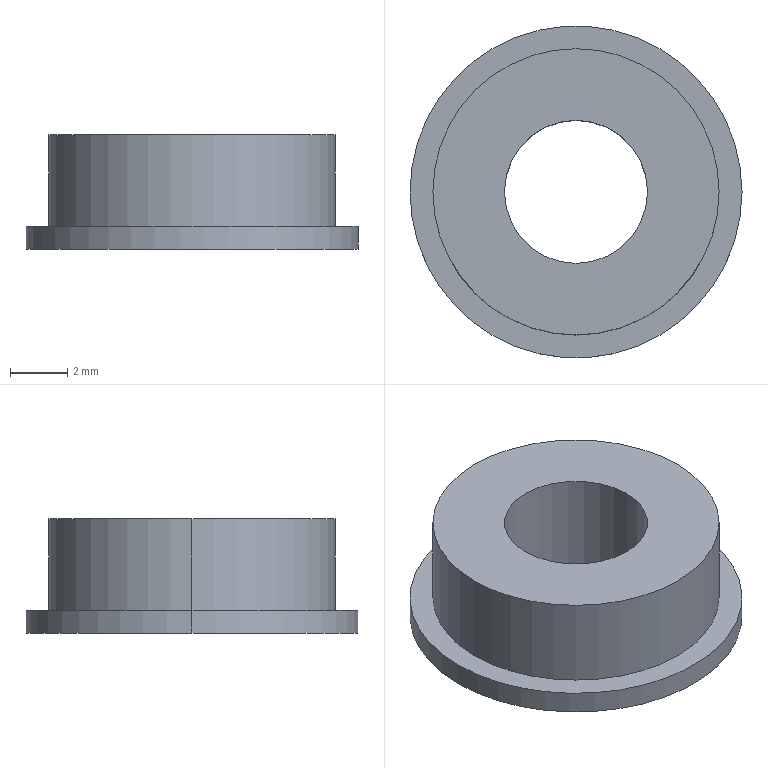Part | SolidWorks | features Extrusion 1, ICE 1 | 1 solid | 9 faces | box 11.6 x 11.6 x 4 mm | volume 257.334 mm3 | cylinder 6 | plane 3 | commonest cylinder face diameters 5 x2 10 x2 11.6 x2
STEP:
#1=CARTESIAN_POINT('',(5.,0.,4.));
#2=VERTEX_POINT('',#1);
#3=CARTESIAN_POINT('',(-5.,0.,4.));
#4=VERTEX_POINT('',#3);
#5=CARTESIAN_POINT('',(0.,0.,4.));
#6=DIRECTION('',(0.,0.,1.));
#7=DIRECTION('',(1.,0.,0.));
#8=AXIS2_PLACEMENT_3D('',#5,#6,#7);
#9=CIRCLE('',#8,5.);
#10=EDGE_CURVE('',#2,#4,#9,.T.);
#11=ORIENTED_EDGE('',*,*,#10,.F.);
#12=CARTESIAN_POINT('',(5.,0.,0.8));
#13=VERTEX_POINT('',#12);
#14=CARTESIAN_POINT('',(5.,0.,4.));
#15=DIRECTION('',(0.,0.,-1.));
#16=VECTOR('',#15,1000.);
#17=LINE('',#14,#16);
#18=EDGE_CURVE('',#2,#13,#17,.T.);
#19=ORIENTED_EDGE('',*,*,#18,.T.);
#20=CARTESIAN_POINT('',(-5.,0.,0.8));
#21=VERTEX_POINT('',#20);
#22=CARTESIAN_POINT('',(0.,0.,0.8));
#23=DIRECTION('',(0.,0.,1.));
#24=DIRECTION('',(1.,0.,0.));
#25=AXIS2_PLACEMENT_3D('',#22,#23,#24);
#26=CIRCLE('',#25,5.);
#27=EDGE_CURVE('',#13,#21,#26,.T.);
#28=ORIENTED_EDGE('',*,*,#27,.T.);
#29=CARTESIAN_POINT('',(-5.,0.,4.));
#30=DIRECTION('',(0.,0.,-1.));
#31=VECTOR('',#30,1000.);
#32=LINE('',#29,#31);
#33=EDGE_CURVE('',#4,#21,#32,.T.);
#34=ORIENTED_EDGE('',*,*,#33,.F.);
#35=EDGE_LOOP('',(#11,#19,#28,#34));
#36=FACE_OUTER_BOUND('',#35,.T.);
#37=CARTESIAN_POINT('',(0.,0.,4.));
#38=DIRECTION('',(0.,0.,-1.));
#39=DIRECTION('',(-1.,0.,0.));
#40=AXIS2_PLACEMENT_3D('',#37,#38,#39);
#41=CYLINDRICAL_SURFACE('',#40,5.);
#42=ADVANCED_FACE('',(#36),#41,.T.);
#43=CARTESIAN_POINT('',(-2.5,0.,4.));
#44=VERTEX_POINT('',#43);
#45=CARTESIAN_POINT('',(2.5,0.,4.));
#46=VERTEX_POINT('',#45);
#47=CARTESIAN_POINT('',(0.,0.,4.));
#48=DIRECTION('',(0.,0.,1.));
#49=DIRECTION('',(1.,0.,0.));
#50=AXIS2_PLACEMENT_3D('',#47,#48,#49);
#51=CIRCLE('',#50,2.5);
#52=EDGE_CURVE('',#44,#46,#51,.T.);
#53=ORIENTED_EDGE('',*,*,#52,.T.);
#54=CARTESIAN_POINT('',(2.5,0.,0.));
#55=VERTEX_POINT('',#54);
#56=CARTESIAN_POINT('',(2.5,0.,0.8));
#57=DIRECTION('',(0.,0.,-1.));
#58=VECTOR('',#57,1000.);
#59=LINE('',#56,#58);
#60=EDGE_CURVE('',#46,#55,#59,.T.);
#61=ORIENTED_EDGE('',*,*,#60,.T.);
#62=CARTESIAN_POINT('',(-2.5,0.,0.));
#63=VERTEX_POINT('',#62);
#64=CARTESIAN_POINT('',(0.,0.,0.));
#65=DIRECTION('',(0.,0.,1.));
#66=DIRECTION('',(1.,0.,0.));
#67=AXIS2_PLACEMENT_3D('',#64,#65,#66);
#68=CIRCLE('',#67,2.5);
#69=EDGE_CURVE('',#63,#55,#68,.T.);
#70=ORIENTED_EDGE('',*,*,#69,.F.);
#71=CARTESIAN_POINT('',(-2.5,0.,0.8));
#72=DIRECTION('',(0.,0.,-1.));
#73=VECTOR('',#72,1000.);
#74=LINE('',#71,#73);
#75=EDGE_CURVE('',#44,#63,#74,.T.);
#76=ORIENTED_EDGE('',*,*,#75,.F.);
#77=EDGE_LOOP('',(#53,#61,#70,#76));
#78=FACE_OUTER_BOUND('',#77,.T.);
#79=CARTESIAN_POINT('',(0.,0.,0.8));
#80=DIRECTION('',(0.,0.,-1.));
#81=DIRECTION('',(-1.,0.,0.));
#82=AXIS2_PLACEMENT_3D('',#79,#80,#81);
#83=CYLINDRICAL_SURFACE('',#82,2.5);
#84=ADVANCED_FACE('',(#78),#83,.F.);
#85=CARTESIAN_POINT('',(5.8,0.,0.8));
#86=VERTEX_POINT('',#85);
#87=CARTESIAN_POINT('',(-5.8,0.,0.8));
#88=VERTEX_POINT('',#87);
#89=CARTESIAN_POINT('',(0.,0.,0.8));
#90=DIRECTION('',(0.,0.,1.));
#91=DIRECTION('',(1.,0.,0.));
#92=AXIS2_PLACEMENT_3D('',#89,#90,#91);
#93=CIRCLE('',#92,5.8);
#94=EDGE_CURVE('',#86,#88,#93,.T.);
#95=ORIENTED_EDGE('',*,*,#94,.F.);
#96=CARTESIAN_POINT('',(5.8,0.,0.));
#97=VERTEX_POINT('',#96);
#98=CARTESIAN_POINT('',(5.8,0.,0.8));
#99=DIRECTION('',(0.,0.,-1.));
#100=VECTOR('',#99,1000.);
#101=LINE('',#98,#100);
#102=EDGE_CURVE('',#86,#97,#101,.T.);
#103=ORIENTED_EDGE('',*,*,#102,.T.);
#104=CARTESIAN_POINT('',(-5.8,0.,0.));
#105=VERTEX_POINT('',#104);
#106=CARTESIAN_POINT('',(0.,0.,0.));
#107=DIRECTION('',(0.,0.,1.));
#108=DIRECTION('',(1.,0.,0.));
#109=AXIS2_PLACEMENT_3D('',#106,#107,#108);
#110=CIRCLE('',#109,5.8);
#111=EDGE_CURVE('',#97,#105,#110,.T.);
#112=ORIENTED_EDGE('',*,*,#111,.T.);
#113=CARTESIAN_POINT('',(-5.8,0.,0.8));
#114=DIRECTION('',(0.,0.,-1.));
#115=VECTOR('',#114,1000.);
#116=LINE('',#113,#115);
#117=EDGE_CURVE('',#88,#105,#116,.T.);
#118=ORIENTED_EDGE('',*,*,#117,.F.);
#119=EDGE_LOOP('',(#95,#103,#112,#118));
#120=FACE_OUTER_BOUND('',#119,.T.);
#121=CARTESIAN_POINT('',(0.,0.,0.8));
#122=DIRECTION('',(0.,0.,-1.));
#123=DIRECTION('',(-1.,0.,0.));
#124=AXIS2_PLACEMENT_3D('',#121,#122,#123);
#125=CYLINDRICAL_SURFACE('',#124,5.8);
#126=ADVANCED_FACE('',(#120),#125,.T.);
#127=CARTESIAN_POINT('',(0.,0.,0.8));
#128=DIRECTION('',(0.,0.,1.));
#129=DIRECTION('',(1.,0.,0.));
#130=AXIS2_PLACEMENT_3D('',#127,#128,#129);
#131=CIRCLE('',#130,5.);
#132=EDGE_CURVE('',#21,#13,#131,.T.);
#133=ORIENTED_EDGE('',*,*,#132,.F.);
#134=ORIENTED_EDGE('',*,*,#27,.F.);
#135=EDGE_LOOP('',(#133,#134));
#136=FACE_BOUND('',#135,.T.);
#137=CARTESIAN_POINT('',(0.,0.,0.8));
#138=DIRECTION('',(0.,0.,1.));
#139=DIRECTION('',(1.,0.,0.));
#140=AXIS2_PLACEMENT_3D('',#137,#138,#139);
#141=CIRCLE('',#140,5.8);
#142=EDGE_CURVE('',#88,#86,#141,.T.);
#143=ORIENTED_EDGE('',*,*,#142,.T.);
#144=ORIENTED_EDGE('',*,*,#94,.T.);
#145=EDGE_LOOP('',(#143,#144));
#146=FACE_OUTER_BOUND('',#145,.T.);
#147=CARTESIAN_POINT('',(0.,0.,0.8));
#148=DIRECTION('',(0.,0.,1.));
#149=DIRECTION('',(1.,0.,0.));
#150=AXIS2_PLACEMENT_3D('',#147,#148,#149);
#151=PLANE('',#150);
#152=ADVANCED_FACE('',(#136,#146),#151,.T.);
#153=CARTESIAN_POINT('',(0.,0.,0.));
#154=DIRECTION('',(0.,0.,1.));
#155=DIRECTION('',(1.,0.,0.));
#156=AXIS2_PLACEMENT_3D('',#153,#154,#155);
#157=CIRCLE('',#156,5.8);
#158=EDGE_CURVE('',#105,#97,#157,.T.);
#159=ORIENTED_EDGE('',*,*,#158,.F.);
#160=ORIENTED_EDGE('',*,*,#111,.F.);
#161=EDGE_LOOP('',(#159,#160));
#162=FACE_OUTER_BOUND('',#161,.T.);
#163=ORIENTED_EDGE('',*,*,#69,.T.);
#164=CARTESIAN_POINT('',(0.,0.,0.));
#165=DIRECTION('',(0.,0.,1.));
#166=DIRECTION('',(1.,0.,0.));
#167=AXIS2_PLACEMENT_3D('',#164,#165,#166);
#168=CIRCLE('',#167,2.5);
#169=EDGE_CURVE('',#55,#63,#168,.T.);
#170=ORIENTED_EDGE('',*,*,#169,.T.);
#171=EDGE_LOOP('',(#163,#170));
#172=FACE_BOUND('',#171,.T.);
#173=CARTESIAN_POINT('',(0.,0.,0.));
#174=DIRECTION('',(0.,0.,1.));
#175=DIRECTION('',(1.,0.,0.));
#176=AXIS2_PLACEMENT_3D('',#173,#174,#175);
#177=PLANE('',#176);
#178=ADVANCED_FACE('',(#162,#172),#177,.F.);
#179=ORIENTED_EDGE('',*,*,#102,.F.);
#180=ORIENTED_EDGE('',*,*,#142,.F.);
#181=ORIENTED_EDGE('',*,*,#117,.T.);
#182=ORIENTED_EDGE('',*,*,#158,.T.);
#183=EDGE_LOOP('',(#179,#180,#181,#182));
#184=FACE_OUTER_BOUND('',#183,.T.);
#185=CARTESIAN_POINT('',(0.,0.,0.8));
#186=DIRECTION('',(0.,0.,-1.));
#187=DIRECTION('',(-1.,0.,0.));
#188=AXIS2_PLACEMENT_3D('',#185,#186,#187);
#189=CYLINDRICAL_SURFACE('',#188,5.8);
#190=ADVANCED_FACE('',(#184),#189,.T.);
#191=ORIENTED_EDGE('',*,*,#60,.F.);
#192=CARTESIAN_POINT('',(0.,0.,4.));
#193=DIRECTION('',(0.,0.,1.));
#194=DIRECTION('',(1.,0.,0.));
#195=AXIS2_PLACEMENT_3D('',#192,#193,#194);
#196=CIRCLE('',#195,2.5);
#197=EDGE_CURVE('',#46,#44,#196,.T.);
#198=ORIENTED_EDGE('',*,*,#197,.T.);
#199=ORIENTED_EDGE('',*,*,#75,.T.);
#200=ORIENTED_EDGE('',*,*,#169,.F.);
#201=EDGE_LOOP('',(#191,#198,#199,#200));
#202=FACE_OUTER_BOUND('',#201,.T.);
#203=CARTESIAN_POINT('',(0.,0.,0.8));
#204=DIRECTION('',(0.,0.,-1.));
#205=DIRECTION('',(-1.,0.,0.));
#206=AXIS2_PLACEMENT_3D('',#203,#204,#205);
#207=CYLINDRICAL_SURFACE('',#206,2.5);
#208=ADVANCED_FACE('',(#202),#207,.F.);
#209=CARTESIAN_POINT('',(0.,0.,4.));
#210=DIRECTION('',(0.,0.,1.));
#211=DIRECTION('',(1.,0.,0.));
#212=AXIS2_PLACEMENT_3D('',#209,#210,#211);
#213=CIRCLE('',#212,5.);
#214=EDGE_CURVE('',#4,#2,#213,.T.);
#215=ORIENTED_EDGE('',*,*,#214,.T.);
#216=ORIENTED_EDGE('',*,*,#10,.T.);
#217=EDGE_LOOP('',(#215,#216));
#218=FACE_OUTER_BOUND('',#217,.T.);
#219=ORIENTED_EDGE('',*,*,#52,.F.);
#220=ORIENTED_EDGE('',*,*,#197,.F.);
#221=EDGE_LOOP('',(#219,#220));
#222=FACE_BOUND('',#221,.T.);
#223=CARTESIAN_POINT('',(0.,0.,4.));
#224=DIRECTION('',(0.,0.,1.));
#225=DIRECTION('',(1.,0.,0.));
#226=AXIS2_PLACEMENT_3D('',#223,#224,#225);
#227=PLANE('',#226);
#228=ADVANCED_FACE('',(#218,#222),#227,.T.);
#229=ORIENTED_EDGE('',*,*,#18,.F.);
#230=ORIENTED_EDGE('',*,*,#214,.F.);
#231=ORIENTED_EDGE('',*,*,#33,.T.);
#232=ORIENTED_EDGE('',*,*,#132,.T.);
#233=EDGE_LOOP('',(#229,#230,#231,#232));
#234=FACE_OUTER_BOUND('',#233,.T.);
#235=CARTESIAN_POINT('',(0.,0.,4.));
#236=DIRECTION('',(0.,0.,-1.));
#237=DIRECTION('',(-1.,0.,0.));
#238=AXIS2_PLACEMENT_3D('',#235,#236,#237);
#239=CYLINDRICAL_SURFACE('',#238,5.);
#240=ADVANCED_FACE('',(#234),#239,.T.);
#241=CLOSED_SHELL('',(#42,#84,#126,#152,#178,#190,#208,#228,#240));
#242=MANIFOLD_SOLID_BREP('',#241);
#243=CARTESIAN_POINT('',(0.,0.,0.));
#244=DIRECTION('',(0.,0.,1.));
#245=DIRECTION('',(1.,0.,0.));
#246=AXIS2_PLACEMENT_3D('',#243,#244,#245);
#247=(LENGTH_UNIT()NAMED_UNIT(*)SI_UNIT(.MILLI.,.METRE.));
#248=UNCERTAINTY_MEASURE_WITH_UNIT(LENGTH_MEASURE(0.00001),#247,'','');
#249=(NAMED_UNIT(*)PLANE_ANGLE_UNIT()SI_UNIT($,.RADIAN.));
#250=(NAMED_UNIT(*)SI_UNIT($,.STERADIAN.)SOLID_ANGLE_UNIT());
#251=(GEOMETRIC_REPRESENTATION_CONTEXT(3)GLOBAL_UNCERTAINTY_ASSIGNED_CONTEXT((#248))GLOBAL_UNIT_ASSIGNED_CONTEXT((#247,#249,#250))REPRESENTATION_CONTEXT('',''));
#252=ADVANCED_BREP_SHAPE_REPRESENTATION('',(#242,#246),#251);